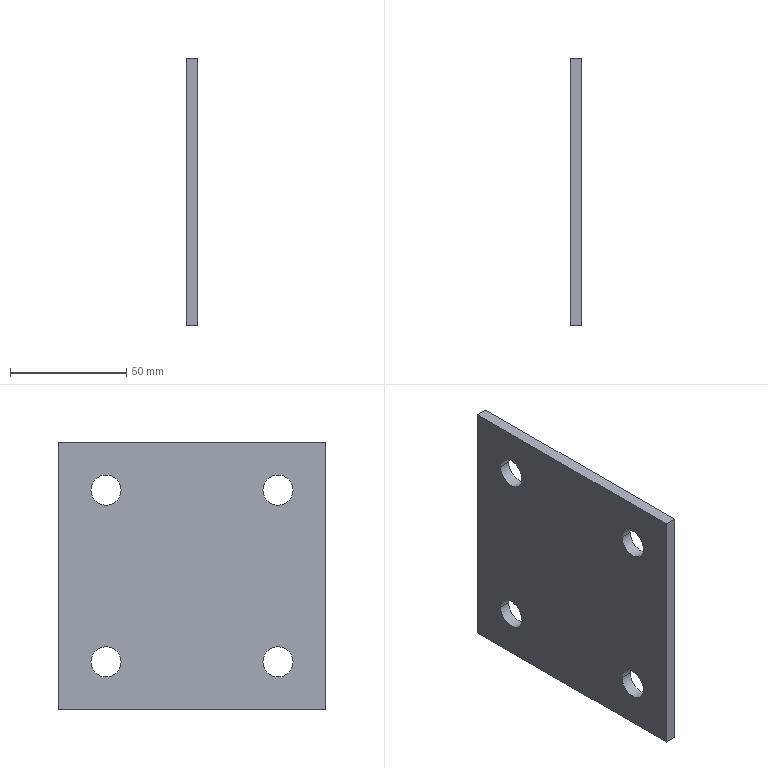Part | STEP file | 09-38 Cylinder pad plate | 1 solid | 14 faces | box 5 x 115 x 115 mm | volume 63470 mm3 | cylinder 8 | plane 6 | commonest cylinder face diameters 13 x8
STEP:
#1=CARTESIAN_POINT('',(0.,0.,0.));
#2=DIRECTION('',(0.,0.,1.));
#3=DIRECTION('',(1.,0.,0.));
#4=AXIS2_PLACEMENT_3D('',#1,#2,#3);
#5=CARTESIAN_POINT('',(5.,-43.5,37.));
#6=VERTEX_POINT('',#5);
#7=CARTESIAN_POINT('',(0.,-43.5,37.));
#8=VERTEX_POINT('',#7);
#9=CARTESIAN_POINT('',(5.,-43.5,37.));
#10=DIRECTION('',(-1.,0.,0.));
#11=VECTOR('',#10,1.);
#12=LINE('',#9,#11);
#13=CARTESIAN_POINT('',(5.,-37.,37.));
#14=DIRECTION('',(-1.,0.,0.));
#15=DIRECTION('',(0.,-1.,0.));
#16=AXIS2_PLACEMENT_3D('',#13,#14,#15);
#17=CYLINDRICAL_SURFACE('',#16,6.5);
#18=CARTESIAN_POINT('',(6.283,0.));
#19=DIRECTION('',(0.,1.));
#20=VECTOR('',#19,1.);
#21=LINE('',#18,#20);
#22=(GEOMETRIC_REPRESENTATION_CONTEXT(2)PARAMETRIC_REPRESENTATION_CONTEXT()REPRESENTATION_CONTEXT('',''));
#23=DEFINITIONAL_REPRESENTATION('',(#21),#22);
#24=PCURVE('',#17,#23);
#25=CARTESIAN_POINT('',(5.,-37.,37.));
#26=DIRECTION('',(-1.,0.,0.));
#27=DIRECTION('',(0.,-1.,0.));
#28=AXIS2_PLACEMENT_3D('',#25,#26,#27);
#29=CYLINDRICAL_SURFACE('',#28,6.5);
#30=CARTESIAN_POINT('',(0.,0.));
#31=DIRECTION('',(0.,1.));
#32=VECTOR('',#31,1.);
#33=LINE('',#30,#32);
#34=(GEOMETRIC_REPRESENTATION_CONTEXT(2)PARAMETRIC_REPRESENTATION_CONTEXT()REPRESENTATION_CONTEXT('',''));
#35=DEFINITIONAL_REPRESENTATION('',(#33),#34);
#36=PCURVE('',#29,#35);
#37=SURFACE_CURVE('',#12,(#24,#36),.PCURVE_S1.);
#38=EDGE_CURVE('',#6,#8,#37,.T.);
#39=ORIENTED_EDGE('',*,*,#38,.T.);
#40=CARTESIAN_POINT('',(0.,-30.5,37.));
#41=VERTEX_POINT('',#40);
#42=CARTESIAN_POINT('',(0.,-37.,37.));
#43=DIRECTION('',(-1.,0.,0.));
#44=DIRECTION('',(0.,-1.,0.));
#45=AXIS2_PLACEMENT_3D('',#42,#43,#44);
#46=CIRCLE('',#45,6.5);
#47=CARTESIAN_POINT('',(0.,5.));
#48=DIRECTION('',(1.,0.));
#49=VECTOR('',#48,1.);
#50=LINE('',#47,#49);
#51=(GEOMETRIC_REPRESENTATION_CONTEXT(2)PARAMETRIC_REPRESENTATION_CONTEXT()REPRESENTATION_CONTEXT('',''));
#52=DEFINITIONAL_REPRESENTATION('',(#50),#51);
#53=PCURVE('',#17,#52);
#54=CARTESIAN_POINT('',(0.,-57.5,-57.5));
#55=DIRECTION('',(-1.,0.,0.));
#56=DIRECTION('',(0.,0.,1.));
#57=AXIS2_PLACEMENT_3D('',#54,#55,#56);
#58=PLANE('',#57);
#59=CARTESIAN_POINT('',(94.5,20.5));
#60=DIRECTION('',(0.,-1.));
#61=AXIS2_PLACEMENT_2D('',#59,#60);
#62=CIRCLE('',#61,6.5);
#63=(GEOMETRIC_REPRESENTATION_CONTEXT(2)PARAMETRIC_REPRESENTATION_CONTEXT()REPRESENTATION_CONTEXT('',''));
#64=DEFINITIONAL_REPRESENTATION('',(#62),#63);
#65=PCURVE('',#58,#64);
#66=SURFACE_CURVE('',#46,(#53,#65),.PCURVE_S1.);
#67=EDGE_CURVE('',#41,#8,#66,.T.);
#68=ORIENTED_EDGE('',*,*,#67,.F.);
#69=CARTESIAN_POINT('',(5.,-30.5,37.));
#70=VERTEX_POINT('',#69);
#71=CARTESIAN_POINT('',(5.,-30.5,37.));
#72=DIRECTION('',(-1.,0.,0.));
#73=VECTOR('',#72,1.);
#74=LINE('',#71,#73);
#75=CARTESIAN_POINT('',(3.142,0.));
#76=DIRECTION('',(0.,1.));
#77=VECTOR('',#76,1.);
#78=LINE('',#75,#77);
#79=(GEOMETRIC_REPRESENTATION_CONTEXT(2)PARAMETRIC_REPRESENTATION_CONTEXT()REPRESENTATION_CONTEXT('',''));
#80=DEFINITIONAL_REPRESENTATION('',(#78),#79);
#81=PCURVE('',#17,#80);
#82=CARTESIAN_POINT('',(3.142,0.));
#83=DIRECTION('',(0.,1.));
#84=VECTOR('',#83,1.);
#85=LINE('',#82,#84);
#86=(GEOMETRIC_REPRESENTATION_CONTEXT(2)PARAMETRIC_REPRESENTATION_CONTEXT()REPRESENTATION_CONTEXT('',''));
#87=DEFINITIONAL_REPRESENTATION('',(#85),#86);
#88=PCURVE('',#29,#87);
#89=SURFACE_CURVE('',#74,(#81,#88),.PCURVE_S1.);
#90=EDGE_CURVE('',#70,#41,#89,.T.);
#91=ORIENTED_EDGE('',*,*,#90,.F.);
#92=CARTESIAN_POINT('',(5.,-37.,37.));
#93=DIRECTION('',(1.,0.,0.));
#94=DIRECTION('',(0.,-1.,0.));
#95=AXIS2_PLACEMENT_3D('',#92,#93,#94);
#96=CIRCLE('',#95,6.5);
#97=CARTESIAN_POINT('',(6.283,0.));
#98=DIRECTION('',(-1.,0.));
#99=VECTOR('',#98,1.);
#100=LINE('',#97,#99);
#101=(GEOMETRIC_REPRESENTATION_CONTEXT(2)PARAMETRIC_REPRESENTATION_CONTEXT()REPRESENTATION_CONTEXT('',''));
#102=DEFINITIONAL_REPRESENTATION('',(#100),#101);
#103=PCURVE('',#17,#102);
#104=CARTESIAN_POINT('',(5.,-57.5,-57.5));
#105=DIRECTION('',(-1.,0.,0.));
#106=DIRECTION('',(0.,0.,1.));
#107=AXIS2_PLACEMENT_3D('',#104,#105,#106);
#108=PLANE('',#107);
#109=CARTESIAN_POINT('',(94.5,14.));
#110=CARTESIAN_POINT('',(83.242,14.));
#111=CARTESIAN_POINT('',(88.871,23.75));
#112=CARTESIAN_POINT('',(94.5,33.5));
#113=CARTESIAN_POINT('',(100.129,23.75));
#114=CARTESIAN_POINT('',(105.758,14.));
#115=CARTESIAN_POINT('',(94.5,14.));
#116=(BOUNDED_CURVE()B_SPLINE_CURVE(2,(#109,#110,#111,#112,#113,#114,#115),.UNSPECIFIED.,.T.,.F.)B_SPLINE_CURVE_WITH_KNOTS((1,2,2,2,2,1),(-2.094,0.,2.094,4.189,6.283,8.378),.UNSPECIFIED.)CURVE()GEOMETRIC_REPRESENTATION_ITEM()RATIONAL_B_SPLINE_CURVE((1.,0.5,1.,0.5,1.,0.5,1.))REPRESENTATION_ITEM(''));
#117=(GEOMETRIC_REPRESENTATION_CONTEXT(2)PARAMETRIC_REPRESENTATION_CONTEXT()REPRESENTATION_CONTEXT('',''));
#118=DEFINITIONAL_REPRESENTATION('',(#116),#117);
#119=PCURVE('',#108,#118);
#120=SURFACE_CURVE('',#96,(#103,#119),.PCURVE_S1.);
#121=EDGE_CURVE('',#6,#70,#120,.T.);
#122=ORIENTED_EDGE('',*,*,#121,.F.);
#123=EDGE_LOOP('',(#39,#68,#91,#122));
#124=FACE_BOUND('',#123,.F.);
#125=ADVANCED_FACE('',(#124),#17,.F.);
#126=CARTESIAN_POINT('',(5.,30.5,-37.));
#127=VERTEX_POINT('',#126);
#128=CARTESIAN_POINT('',(0.,30.5,-37.));
#129=VERTEX_POINT('',#128);
#130=CARTESIAN_POINT('',(5.,30.5,-37.));
#131=DIRECTION('',(-1.,0.,0.));
#132=VECTOR('',#131,1.);
#133=LINE('',#130,#132);
#134=CARTESIAN_POINT('',(5.,37.,-37.));
#135=DIRECTION('',(-1.,0.,0.));
#136=DIRECTION('',(0.,-1.,0.));
#137=AXIS2_PLACEMENT_3D('',#134,#135,#136);
#138=CYLINDRICAL_SURFACE('',#137,6.5);
#139=CARTESIAN_POINT('',(6.283,0.));
#140=DIRECTION('',(0.,1.));
#141=VECTOR('',#140,1.);
#142=LINE('',#139,#141);
#143=(GEOMETRIC_REPRESENTATION_CONTEXT(2)PARAMETRIC_REPRESENTATION_CONTEXT()REPRESENTATION_CONTEXT('',''));
#144=DEFINITIONAL_REPRESENTATION('',(#142),#143);
#145=PCURVE('',#138,#144);
#146=CARTESIAN_POINT('',(5.,37.,-37.));
#147=DIRECTION('',(-1.,0.,0.));
#148=DIRECTION('',(0.,-1.,0.));
#149=AXIS2_PLACEMENT_3D('',#146,#147,#148);
#150=CYLINDRICAL_SURFACE('',#149,6.5);
#151=CARTESIAN_POINT('',(0.,0.));
#152=DIRECTION('',(0.,1.));
#153=VECTOR('',#152,1.);
#154=LINE('',#151,#153);
#155=(GEOMETRIC_REPRESENTATION_CONTEXT(2)PARAMETRIC_REPRESENTATION_CONTEXT()REPRESENTATION_CONTEXT('',''));
#156=DEFINITIONAL_REPRESENTATION('',(#154),#155);
#157=PCURVE('',#150,#156);
#158=SURFACE_CURVE('',#133,(#145,#157),.PCURVE_S1.);
#159=EDGE_CURVE('',#127,#129,#158,.T.);
#160=ORIENTED_EDGE('',*,*,#159,.T.);
#161=CARTESIAN_POINT('',(0.,43.5,-37.));
#162=VERTEX_POINT('',#161);
#163=CARTESIAN_POINT('',(0.,37.,-37.));
#164=DIRECTION('',(1.,0.,0.));
#165=DIRECTION('',(0.,-1.,0.));
#166=AXIS2_PLACEMENT_3D('',#163,#164,#165);
#167=CIRCLE('',#166,6.5);
#168=CARTESIAN_POINT('',(6.283,5.));
#169=DIRECTION('',(-1.,0.));
#170=VECTOR('',#169,1.);
#171=LINE('',#168,#170);
#172=(GEOMETRIC_REPRESENTATION_CONTEXT(2)PARAMETRIC_REPRESENTATION_CONTEXT()REPRESENTATION_CONTEXT('',''));
#173=DEFINITIONAL_REPRESENTATION('',(#171),#172);
#174=PCURVE('',#138,#173);
#175=CARTESIAN_POINT('',(20.5,88.));
#176=CARTESIAN_POINT('',(9.242,88.));
#177=CARTESIAN_POINT('',(14.871,97.75));
#178=CARTESIAN_POINT('',(20.5,107.5));
#179=CARTESIAN_POINT('',(26.129,97.75));
#180=CARTESIAN_POINT('',(31.758,88.));
#181=CARTESIAN_POINT('',(20.5,88.));
#182=(BOUNDED_CURVE()B_SPLINE_CURVE(2,(#175,#176,#177,#178,#179,#180,#181),.UNSPECIFIED.,.T.,.F.)B_SPLINE_CURVE_WITH_KNOTS((1,2,2,2,2,1),(-2.094,0.,2.094,4.189,6.283,8.378),.UNSPECIFIED.)CURVE()GEOMETRIC_REPRESENTATION_ITEM()RATIONAL_B_SPLINE_CURVE((1.,0.5,1.,0.5,1.,0.5,1.))REPRESENTATION_ITEM(''));
#183=(GEOMETRIC_REPRESENTATION_CONTEXT(2)PARAMETRIC_REPRESENTATION_CONTEXT()REPRESENTATION_CONTEXT('',''));
#184=DEFINITIONAL_REPRESENTATION('',(#182),#183);
#185=PCURVE('',#58,#184);
#186=SURFACE_CURVE('',#167,(#174,#185),.PCURVE_S1.);
#187=EDGE_CURVE('',#129,#162,#186,.T.);
#188=ORIENTED_EDGE('',*,*,#187,.T.);
#189=CARTESIAN_POINT('',(5.,43.5,-37.));
#190=VERTEX_POINT('',#189);
#191=CARTESIAN_POINT('',(5.,43.5,-37.));
#192=DIRECTION('',(-1.,0.,0.));
#193=VECTOR('',#192,1.);
#194=LINE('',#191,#193);
#195=CARTESIAN_POINT('',(3.142,0.));
#196=DIRECTION('',(0.,1.));
#197=VECTOR('',#196,1.);
#198=LINE('',#195,#197);
#199=(GEOMETRIC_REPRESENTATION_CONTEXT(2)PARAMETRIC_REPRESENTATION_CONTEXT()REPRESENTATION_CONTEXT('',''));
#200=DEFINITIONAL_REPRESENTATION('',(#198),#199);
#201=PCURVE('',#138,#200);
#202=CARTESIAN_POINT('',(3.142,0.));
#203=DIRECTION('',(0.,1.));
#204=VECTOR('',#203,1.);
#205=LINE('',#202,#204);
#206=(GEOMETRIC_REPRESENTATION_CONTEXT(2)PARAMETRIC_REPRESENTATION_CONTEXT()REPRESENTATION_CONTEXT('',''));
#207=DEFINITIONAL_REPRESENTATION('',(#205),#206);
#208=PCURVE('',#150,#207);
#209=SURFACE_CURVE('',#194,(#201,#208),.PCURVE_S1.);
#210=EDGE_CURVE('',#190,#162,#209,.T.);
#211=ORIENTED_EDGE('',*,*,#210,.F.);
#212=CARTESIAN_POINT('',(5.,37.,-37.));
#213=DIRECTION('',(1.,0.,0.));
#214=DIRECTION('',(0.,-1.,0.));
#215=AXIS2_PLACEMENT_3D('',#212,#213,#214);
#216=CIRCLE('',#215,6.5);
#217=CARTESIAN_POINT('',(6.283,0.));
#218=DIRECTION('',(-1.,0.));
#219=VECTOR('',#218,1.);
#220=LINE('',#217,#219);
#221=(GEOMETRIC_REPRESENTATION_CONTEXT(2)PARAMETRIC_REPRESENTATION_CONTEXT()REPRESENTATION_CONTEXT('',''));
#222=DEFINITIONAL_REPRESENTATION('',(#220),#221);
#223=PCURVE('',#138,#222);
#224=CARTESIAN_POINT('',(20.5,88.));
#225=CARTESIAN_POINT('',(9.242,88.));
#226=CARTESIAN_POINT('',(14.871,97.75));
#227=CARTESIAN_POINT('',(20.5,107.5));
#228=CARTESIAN_POINT('',(26.129,97.75));
#229=CARTESIAN_POINT('',(31.758,88.));
#230=CARTESIAN_POINT('',(20.5,88.));
#231=(BOUNDED_CURVE()B_SPLINE_CURVE(2,(#224,#225,#226,#227,#228,#229,#230),.UNSPECIFIED.,.T.,.F.)B_SPLINE_CURVE_WITH_KNOTS((1,2,2,2,2,1),(-2.094,0.,2.094,4.189,6.283,8.378),.UNSPECIFIED.)CURVE()GEOMETRIC_REPRESENTATION_ITEM()RATIONAL_B_SPLINE_CURVE((1.,0.5,1.,0.5,1.,0.5,1.))REPRESENTATION_ITEM(''));
#232=(GEOMETRIC_REPRESENTATION_CONTEXT(2)PARAMETRIC_REPRESENTATION_CONTEXT()REPRESENTATION_CONTEXT('',''));
#233=DEFINITIONAL_REPRESENTATION('',(#231),#232);
#234=PCURVE('',#108,#233);
#235=SURFACE_CURVE('',#216,(#223,#234),.PCURVE_S1.);
#236=EDGE_CURVE('',#127,#190,#235,.T.);
#237=ORIENTED_EDGE('',*,*,#236,.F.);
#238=EDGE_LOOP('',(#160,#188,#211,#237));
#239=FACE_BOUND('',#238,.F.);
#240=ADVANCED_FACE('',(#239),#138,.F.);
#241=CARTESIAN_POINT('',(5.,30.5,37.));
#242=VERTEX_POINT('',#241);
#243=CARTESIAN_POINT('',(0.,30.5,37.));
#244=VERTEX_POINT('',#243);
#245=CARTESIAN_POINT('',(5.,30.5,37.));
#246=DIRECTION('',(-1.,0.,0.));
#247=VECTOR('',#246,1.);
#248=LINE('',#245,#247);
#249=CARTESIAN_POINT('',(5.,37.,37.));
#250=DIRECTION('',(-1.,0.,0.));
#251=DIRECTION('',(0.,-1.,0.));
#252=AXIS2_PLACEMENT_3D('',#249,#250,#251);
#253=CYLINDRICAL_SURFACE('',#252,6.5);
#254=CARTESIAN_POINT('',(6.283,0.));
#255=DIRECTION('',(0.,1.));
#256=VECTOR('',#255,1.);
#257=LINE('',#254,#256);
#258=(GEOMETRIC_REPRESENTATION_CONTEXT(2)PARAMETRIC_REPRESENTATION_CONTEXT()REPRESENTATION_CONTEXT('',''));
#259=DEFINITIONAL_REPRESENTATION('',(#257),#258);
#260=PCURVE('',#253,#259);
#261=CARTESIAN_POINT('',(5.,37.,37.));
#262=DIRECTION('',(-1.,0.,0.));
#263=DIRECTION('',(0.,-1.,0.));
#264=AXIS2_PLACEMENT_3D('',#261,#262,#263);
#265=CYLINDRICAL_SURFACE('',#264,6.5);
#266=CARTESIAN_POINT('',(0.,0.));
#267=DIRECTION('',(0.,1.));
#268=VECTOR('',#267,1.);
#269=LINE('',#266,#268);
#270=(GEOMETRIC_REPRESENTATION_CONTEXT(2)PARAMETRIC_REPRESENTATION_CONTEXT()REPRESENTATION_CONTEXT('',''));
#271=DEFINITIONAL_REPRESENTATION('',(#269),#270);
#272=PCURVE('',#265,#271);
#273=SURFACE_CURVE('',#248,(#260,#272),.PCURVE_S1.);
#274=EDGE_CURVE('',#242,#244,#273,.T.);
#275=ORIENTED_EDGE('',*,*,#274,.T.);
#276=CARTESIAN_POINT('',(0.,43.5,37.));
#277=VERTEX_POINT('',#276);
#278=CARTESIAN_POINT('',(0.,37.,37.));
#279=DIRECTION('',(1.,0.,0.));
#280=DIRECTION('',(0.,-1.,0.));
#281=AXIS2_PLACEMENT_3D('',#278,#279,#280);
#282=CIRCLE('',#281,6.5);
#283=CARTESIAN_POINT('',(6.283,5.));
#284=DIRECTION('',(-1.,0.));
#285=VECTOR('',#284,1.);
#286=LINE('',#283,#285);
#287=(GEOMETRIC_REPRESENTATION_CONTEXT(2)PARAMETRIC_REPRESENTATION_CONTEXT()REPRESENTATION_CONTEXT('',''));
#288=DEFINITIONAL_REPRESENTATION('',(#286),#287);
#289=PCURVE('',#253,#288);
#290=CARTESIAN_POINT('',(94.5,88.));
#291=CARTESIAN_POINT('',(83.242,88.));
#292=CARTESIAN_POINT('',(88.871,97.75));
#293=CARTESIAN_POINT('',(94.5,107.5));
#294=CARTESIAN_POINT('',(100.129,97.75));
#295=CARTESIAN_POINT('',(105.758,88.));
#296=CARTESIAN_POINT('',(94.5,88.));
#297=(BOUNDED_CURVE()B_SPLINE_CURVE(2,(#290,#291,#292,#293,#294,#295,#296),.UNSPECIFIED.,.T.,.F.)B_SPLINE_CURVE_WITH_KNOTS((1,2,2,2,2,1),(-2.094,0.,2.094,4.189,6.283,8.378),.UNSPECIFIED.)CURVE()GEOMETRIC_REPRESENTATION_ITEM()RATIONAL_B_SPLINE_CURVE((1.,0.5,1.,0.5,1.,0.5,1.))REPRESENTATION_ITEM(''));
#298=(GEOMETRIC_REPRESENTATION_CONTEXT(2)PARAMETRIC_REPRESENTATION_CONTEXT()REPRESENTATION_CONTEXT('',''));
#299=DEFINITIONAL_REPRESENTATION('',(#297),#298);
#300=PCURVE('',#58,#299);
#301=SURFACE_CURVE('',#282,(#289,#300),.PCURVE_S1.);
#302=EDGE_CURVE('',#244,#277,#301,.T.);
#303=ORIENTED_EDGE('',*,*,#302,.T.);
#304=CARTESIAN_POINT('',(5.,43.5,37.));
#305=VERTEX_POINT('',#304);
#306=CARTESIAN_POINT('',(5.,43.5,37.));
#307=DIRECTION('',(-1.,0.,0.));
#308=VECTOR('',#307,1.);
#309=LINE('',#306,#308);
#310=CARTESIAN_POINT('',(3.142,0.));
#311=DIRECTION('',(0.,1.));
#312=VECTOR('',#311,1.);
#313=LINE('',#310,#312);
#314=(GEOMETRIC_REPRESENTATION_CONTEXT(2)PARAMETRIC_REPRESENTATION_CONTEXT()REPRESENTATION_CONTEXT('',''));
#315=DEFINITIONAL_REPRESENTATION('',(#313),#314);
#316=PCURVE('',#253,#315);
#317=CARTESIAN_POINT('',(3.142,0.));
#318=DIRECTION('',(0.,1.));
#319=VECTOR('',#318,1.);
#320=LINE('',#317,#319);
#321=(GEOMETRIC_REPRESENTATION_CONTEXT(2)PARAMETRIC_REPRESENTATION_CONTEXT()REPRESENTATION_CONTEXT('',''));
#322=DEFINITIONAL_REPRESENTATION('',(#320),#321);
#323=PCURVE('',#265,#322);
#324=SURFACE_CURVE('',#309,(#316,#323),.PCURVE_S1.);
#325=EDGE_CURVE('',#305,#277,#324,.T.);
#326=ORIENTED_EDGE('',*,*,#325,.F.);
#327=CARTESIAN_POINT('',(5.,37.,37.));
#328=DIRECTION('',(1.,0.,0.));
#329=DIRECTION('',(0.,-1.,0.));
#330=AXIS2_PLACEMENT_3D('',#327,#328,#329);
#331=CIRCLE('',#330,6.5);
#332=CARTESIAN_POINT('',(6.283,0.));
#333=DIRECTION('',(-1.,0.));
#334=VECTOR('',#333,1.);
#335=LINE('',#332,#334);
#336=(GEOMETRIC_REPRESENTATION_CONTEXT(2)PARAMETRIC_REPRESENTATION_CONTEXT()REPRESENTATION_CONTEXT('',''));
#337=DEFINITIONAL_REPRESENTATION('',(#335),#336);
#338=PCURVE('',#253,#337);
#339=CARTESIAN_POINT('',(94.5,88.));
#340=CARTESIAN_POINT('',(83.242,88.));
#341=CARTESIAN_POINT('',(88.871,97.75));
#342=CARTESIAN_POINT('',(94.5,107.5));
#343=CARTESIAN_POINT('',(100.129,97.75));
#344=CARTESIAN_POINT('',(105.758,88.));
#345=CARTESIAN_POINT('',(94.5,88.));
#346=(BOUNDED_CURVE()B_SPLINE_CURVE(2,(#339,#340,#341,#342,#343,#344,#345),.UNSPECIFIED.,.T.,.F.)B_SPLINE_CURVE_WITH_KNOTS((1,2,2,2,2,1),(-2.094,0.,2.094,4.189,6.283,8.378),.UNSPECIFIED.)CURVE()GEOMETRIC_REPRESENTATION_ITEM()RATIONAL_B_SPLINE_CURVE((1.,0.5,1.,0.5,1.,0.5,1.))REPRESENTATION_ITEM(''));
#347=(GEOMETRIC_REPRESENTATION_CONTEXT(2)PARAMETRIC_REPRESENTATION_CONTEXT()REPRESENTATION_CONTEXT('',''));
#348=DEFINITIONAL_REPRESENTATION('',(#346),#347);
#349=PCURVE('',#108,#348);
#350=SURFACE_CURVE('',#331,(#338,#349),.PCURVE_S1.);
#351=EDGE_CURVE('',#242,#305,#350,.T.);
#352=ORIENTED_EDGE('',*,*,#351,.F.);
#353=EDGE_LOOP('',(#275,#303,#326,#352));
#354=FACE_BOUND('',#353,.F.);
#355=ADVANCED_FACE('',(#354),#253,.F.);
#356=CARTESIAN_POINT('',(5.,-43.5,-37.));
#357=VERTEX_POINT('',#356);
#358=CARTESIAN_POINT('',(0.,-43.5,-37.));
#359=VERTEX_POINT('',#358);
#360=CARTESIAN_POINT('',(5.,-43.5,-37.));
#361=DIRECTION('',(-1.,0.,0.));
#362=VECTOR('',#361,1.);
#363=LINE('',#360,#362);
#364=CARTESIAN_POINT('',(5.,-37.,-37.));
#365=DIRECTION('',(-1.,0.,0.));
#366=DIRECTION('',(0.,-1.,0.));
#367=AXIS2_PLACEMENT_3D('',#364,#365,#366);
#368=CYLINDRICAL_SURFACE('',#367,6.5);
#369=CARTESIAN_POINT('',(6.283,0.));
#370=DIRECTION('',(0.,1.));
#371=VECTOR('',#370,1.);
#372=LINE('',#369,#371);
#373=(GEOMETRIC_REPRESENTATION_CONTEXT(2)PARAMETRIC_REPRESENTATION_CONTEXT()REPRESENTATION_CONTEXT('',''));
#374=DEFINITIONAL_REPRESENTATION('',(#372),#373);
#375=PCURVE('',#368,#374);
#376=CARTESIAN_POINT('',(5.,-37.,-37.));
#377=DIRECTION('',(-1.,0.,0.));
#378=DIRECTION('',(0.,-1.,0.));
#379=AXIS2_PLACEMENT_3D('',#376,#377,#378);
#380=CYLINDRICAL_SURFACE('',#379,6.5);
#381=CARTESIAN_POINT('',(0.,0.));
#382=DIRECTION('',(0.,1.));
#383=VECTOR('',#382,1.);
#384=LINE('',#381,#383);
#385=(GEOMETRIC_REPRESENTATION_CONTEXT(2)PARAMETRIC_REPRESENTATION_CONTEXT()REPRESENTATION_CONTEXT('',''));
#386=DEFINITIONAL_REPRESENTATION('',(#384),#385);
#387=PCURVE('',#380,#386);
#388=SURFACE_CURVE('',#363,(#375,#387),.PCURVE_S1.);
#389=EDGE_CURVE('',#357,#359,#388,.T.);
#390=ORIENTED_EDGE('',*,*,#389,.T.);
#391=CARTESIAN_POINT('',(0.,-30.5,-37.));
#392=VERTEX_POINT('',#391);
#393=CARTESIAN_POINT('',(0.,-37.,-37.));
#394=DIRECTION('',(1.,0.,0.));
#395=DIRECTION('',(0.,-1.,0.));
#396=AXIS2_PLACEMENT_3D('',#393,#394,#395);
#397=CIRCLE('',#396,6.5);
#398=CARTESIAN_POINT('',(6.283,5.));
#399=DIRECTION('',(-1.,0.));
#400=VECTOR('',#399,1.);
#401=LINE('',#398,#400);
#402=(GEOMETRIC_REPRESENTATION_CONTEXT(2)PARAMETRIC_REPRESENTATION_CONTEXT()REPRESENTATION_CONTEXT('',''));
#403=DEFINITIONAL_REPRESENTATION('',(#401),#402);
#404=PCURVE('',#368,#403);
#405=CARTESIAN_POINT('',(20.5,14.));
#406=CARTESIAN_POINT('',(9.242,14.));
#407=CARTESIAN_POINT('',(14.871,23.75));
#408=CARTESIAN_POINT('',(20.5,33.5));
#409=CARTESIAN_POINT('',(26.129,23.75));
#410=CARTESIAN_POINT('',(31.758,14.));
#411=CARTESIAN_POINT('',(20.5,14.));
#412=(BOUNDED_CURVE()B_SPLINE_CURVE(2,(#405,#406,#407,#408,#409,#410,#411),.UNSPECIFIED.,.T.,.F.)B_SPLINE_CURVE_WITH_KNOTS((1,2,2,2,2,1),(-2.094,0.,2.094,4.189,6.283,8.378),.UNSPECIFIED.)CURVE()GEOMETRIC_REPRESENTATION_ITEM()RATIONAL_B_SPLINE_CURVE((1.,0.5,1.,0.5,1.,0.5,1.))REPRESENTATION_ITEM(''));
#413=(GEOMETRIC_REPRESENTATION_CONTEXT(2)PARAMETRIC_REPRESENTATION_CONTEXT()REPRESENTATION_CONTEXT('',''));
#414=DEFINITIONAL_REPRESENTATION('',(#412),#413);
#415=PCURVE('',#58,#414);
#416=SURFACE_CURVE('',#397,(#404,#415),.PCURVE_S1.);
#417=EDGE_CURVE('',#359,#392,#416,.T.);
#418=ORIENTED_EDGE('',*,*,#417,.T.);
#419=CARTESIAN_POINT('',(5.,-30.5,-37.));
#420=VERTEX_POINT('',#419);
#421=CARTESIAN_POINT('',(5.,-30.5,-37.));
#422=DIRECTION('',(-1.,0.,0.));
#423=VECTOR('',#422,1.);
#424=LINE('',#421,#423);
#425=CARTESIAN_POINT('',(3.142,0.));
#426=DIRECTION('',(0.,1.));
#427=VECTOR('',#426,1.);
#428=LINE('',#425,#427);
#429=(GEOMETRIC_REPRESENTATION_CONTEXT(2)PARAMETRIC_REPRESENTATION_CONTEXT()REPRESENTATION_CONTEXT('',''));
#430=DEFINITIONAL_REPRESENTATION('',(#428),#429);
#431=PCURVE('',#368,#430);
#432=CARTESIAN_POINT('',(3.142,0.));
#433=DIRECTION('',(0.,1.));
#434=VECTOR('',#433,1.);
#435=LINE('',#432,#434);
#436=(GEOMETRIC_REPRESENTATION_CONTEXT(2)PARAMETRIC_REPRESENTATION_CONTEXT()REPRESENTATION_CONTEXT('',''));
#437=DEFINITIONAL_REPRESENTATION('',(#435),#436);
#438=PCURVE('',#380,#437);
#439=SURFACE_CURVE('',#424,(#431,#438),.PCURVE_S1.);
#440=EDGE_CURVE('',#420,#392,#439,.T.);
#441=ORIENTED_EDGE('',*,*,#440,.F.);
#442=CARTESIAN_POINT('',(5.,-37.,-37.));
#443=DIRECTION('',(1.,0.,0.));
#444=DIRECTION('',(0.,-1.,0.));
#445=AXIS2_PLACEMENT_3D('',#442,#443,#444);
#446=CIRCLE('',#445,6.5);
#447=CARTESIAN_POINT('',(6.283,0.));
#448=DIRECTION('',(-1.,0.));
#449=VECTOR('',#448,1.);
#450=LINE('',#447,#449);
#451=(GEOMETRIC_REPRESENTATION_CONTEXT(2)PARAMETRIC_REPRESENTATION_CONTEXT()REPRESENTATION_CONTEXT('',''));
#452=DEFINITIONAL_REPRESENTATION('',(#450),#451);
#453=PCURVE('',#368,#452);
#454=CARTESIAN_POINT('',(20.5,14.));
#455=CARTESIAN_POINT('',(9.242,14.));
#456=CARTESIAN_POINT('',(14.871,23.75));
#457=CARTESIAN_POINT('',(20.5,33.5));
#458=CARTESIAN_POINT('',(26.129,23.75));
#459=CARTESIAN_POINT('',(31.758,14.));
#460=CARTESIAN_POINT('',(20.5,14.));
#461=(BOUNDED_CURVE()B_SPLINE_CURVE(2,(#454,#455,#456,#457,#458,#459,#460),.UNSPECIFIED.,.T.,.F.)B_SPLINE_CURVE_WITH_KNOTS((1,2,2,2,2,1),(-2.094,0.,2.094,4.189,6.283,8.378),.UNSPECIFIED.)CURVE()GEOMETRIC_REPRESENTATION_ITEM()RATIONAL_B_SPLINE_CURVE((1.,0.5,1.,0.5,1.,0.5,1.))REPRESENTATION_ITEM(''));
#462=(GEOMETRIC_REPRESENTATION_CONTEXT(2)PARAMETRIC_REPRESENTATION_CONTEXT()REPRESENTATION_CONTEXT('',''));
#463=DEFINITIONAL_REPRESENTATION('',(#461),#462);
#464=PCURVE('',#108,#463);
#465=SURFACE_CURVE('',#446,(#453,#464),.PCURVE_S1.);
#466=EDGE_CURVE('',#357,#420,#465,.T.);
#467=ORIENTED_EDGE('',*,*,#466,.F.);
#468=EDGE_LOOP('',(#390,#418,#441,#467));
#469=FACE_BOUND('',#468,.F.);
#470=ADVANCED_FACE('',(#469),#368,.F.);
#471=CARTESIAN_POINT('',(0.,-37.,37.));
#472=DIRECTION('',(-1.,0.,0.));
#473=DIRECTION('',(0.,-1.,0.));
#474=AXIS2_PLACEMENT_3D('',#471,#472,#473);
#475=CIRCLE('',#474,6.5);
#476=CARTESIAN_POINT('',(0.,5.));
#477=DIRECTION('',(1.,0.));
#478=VECTOR('',#477,1.);
#479=LINE('',#476,#478);
#480=(GEOMETRIC_REPRESENTATION_CONTEXT(2)PARAMETRIC_REPRESENTATION_CONTEXT()REPRESENTATION_CONTEXT('',''));
#481=DEFINITIONAL_REPRESENTATION('',(#479),#480);
#482=PCURVE('',#29,#481);
#483=CARTESIAN_POINT('',(94.5,20.5));
#484=DIRECTION('',(0.,-1.));
#485=AXIS2_PLACEMENT_2D('',#483,#484);
#486=CIRCLE('',#485,6.5);
#487=(GEOMETRIC_REPRESENTATION_CONTEXT(2)PARAMETRIC_REPRESENTATION_CONTEXT()REPRESENTATION_CONTEXT('',''));
#488=DEFINITIONAL_REPRESENTATION('',(#486),#487);
#489=PCURVE('',#58,#488);
#490=SURFACE_CURVE('',#475,(#482,#489),.PCURVE_S1.);
#491=EDGE_CURVE('',#8,#41,#490,.T.);
#492=ORIENTED_EDGE('',*,*,#491,.F.);
#493=ORIENTED_EDGE('',*,*,#38,.F.);
#494=CARTESIAN_POINT('',(5.,-37.,37.));
#495=DIRECTION('',(1.,0.,0.));
#496=DIRECTION('',(0.,-1.,0.));
#497=AXIS2_PLACEMENT_3D('',#494,#495,#496);
#498=CIRCLE('',#497,6.5);
#499=CARTESIAN_POINT('',(6.283,0.));
#500=DIRECTION('',(-1.,0.));
#501=VECTOR('',#500,1.);
#502=LINE('',#499,#501);
#503=(GEOMETRIC_REPRESENTATION_CONTEXT(2)PARAMETRIC_REPRESENTATION_CONTEXT()REPRESENTATION_CONTEXT('',''));
#504=DEFINITIONAL_REPRESENTATION('',(#502),#503);
#505=PCURVE('',#29,#504);
#506=CARTESIAN_POINT('',(94.5,14.));
#507=CARTESIAN_POINT('',(83.242,14.));
#508=CARTESIAN_POINT('',(88.871,23.75));
#509=CARTESIAN_POINT('',(94.5,33.5));
#510=CARTESIAN_POINT('',(100.129,23.75));
#511=CARTESIAN_POINT('',(105.758,14.));
#512=CARTESIAN_POINT('',(94.5,14.));
#513=(BOUNDED_CURVE()B_SPLINE_CURVE(2,(#506,#507,#508,#509,#510,#511,#512),.UNSPECIFIED.,.T.,.F.)B_SPLINE_CURVE_WITH_KNOTS((1,2,2,2,2,1),(-2.094,0.,2.094,4.189,6.283,8.378),.UNSPECIFIED.)CURVE()GEOMETRIC_REPRESENTATION_ITEM()RATIONAL_B_SPLINE_CURVE((1.,0.5,1.,0.5,1.,0.5,1.))REPRESENTATION_ITEM(''));
#514=(GEOMETRIC_REPRESENTATION_CONTEXT(2)PARAMETRIC_REPRESENTATION_CONTEXT()REPRESENTATION_CONTEXT('',''));
#515=DEFINITIONAL_REPRESENTATION('',(#513),#514);
#516=PCURVE('',#108,#515);
#517=SURFACE_CURVE('',#498,(#505,#516),.PCURVE_S1.);
#518=EDGE_CURVE('',#70,#6,#517,.T.);
#519=ORIENTED_EDGE('',*,*,#518,.F.);
#520=ORIENTED_EDGE('',*,*,#90,.T.);
#521=EDGE_LOOP('',(#492,#493,#519,#520));
#522=FACE_BOUND('',#521,.F.);
#523=ADVANCED_FACE('',(#522),#29,.F.);
#524=ORIENTED_EDGE('',*,*,#491,.F.);
#525=ORIENTED_EDGE('',*,*,#67,.F.);
#526=EDGE_LOOP('',(#524,#525));
#527=FACE_BOUND('',#526,.T.);
#528=ORIENTED_EDGE('',*,*,#187,.T.);
#529=CARTESIAN_POINT('',(0.,37.,-37.));
#530=DIRECTION('',(1.,0.,0.));
#531=DIRECTION('',(0.,-1.,0.));
#532=AXIS2_PLACEMENT_3D('',#529,#530,#531);
#533=CIRCLE('',#532,6.5);
#534=CARTESIAN_POINT('',(20.5,88.));
#535=CARTESIAN_POINT('',(9.242,88.));
#536=CARTESIAN_POINT('',(14.871,97.75));
#537=CARTESIAN_POINT('',(20.5,107.5));
#538=CARTESIAN_POINT('',(26.129,97.75));
#539=CARTESIAN_POINT('',(31.758,88.));
#540=CARTESIAN_POINT('',(20.5,88.));
#541=(BOUNDED_CURVE()B_SPLINE_CURVE(2,(#534,#535,#536,#537,#538,#539,#540),.UNSPECIFIED.,.T.,.F.)B_SPLINE_CURVE_WITH_KNOTS((1,2,2,2,2,1),(-2.094,0.,2.094,4.189,6.283,8.378),.UNSPECIFIED.)CURVE()GEOMETRIC_REPRESENTATION_ITEM()RATIONAL_B_SPLINE_CURVE((1.,0.5,1.,0.5,1.,0.5,1.))REPRESENTATION_ITEM(''));
#542=(GEOMETRIC_REPRESENTATION_CONTEXT(2)PARAMETRIC_REPRESENTATION_CONTEXT()REPRESENTATION_CONTEXT('',''));
#543=DEFINITIONAL_REPRESENTATION('',(#541),#542);
#544=PCURVE('',#58,#543);
#545=CARTESIAN_POINT('',(6.283,5.));
#546=DIRECTION('',(-1.,0.));
#547=VECTOR('',#546,1.);
#548=LINE('',#545,#547);
#549=(GEOMETRIC_REPRESENTATION_CONTEXT(2)PARAMETRIC_REPRESENTATION_CONTEXT()REPRESENTATION_CONTEXT('',''));
#550=DEFINITIONAL_REPRESENTATION('',(#548),#549);
#551=PCURVE('',#150,#550);
#552=SURFACE_CURVE('',#533,(#544,#551),.PCURVE_S1.);
#553=EDGE_CURVE('',#162,#129,#552,.T.);
#554=ORIENTED_EDGE('',*,*,#553,.T.);
#555=EDGE_LOOP('',(#528,#554));
#556=FACE_BOUND('',#555,.T.);
#557=ORIENTED_EDGE('',*,*,#302,.T.);
#558=CARTESIAN_POINT('',(0.,37.,37.));
#559=DIRECTION('',(1.,0.,0.));
#560=DIRECTION('',(0.,-1.,0.));
#561=AXIS2_PLACEMENT_3D('',#558,#559,#560);
#562=CIRCLE('',#561,6.5);
#563=CARTESIAN_POINT('',(94.5,88.));
#564=CARTESIAN_POINT('',(83.242,88.));
#565=CARTESIAN_POINT('',(88.871,97.75));
#566=CARTESIAN_POINT('',(94.5,107.5));
#567=CARTESIAN_POINT('',(100.129,97.75));
#568=CARTESIAN_POINT('',(105.758,88.));
#569=CARTESIAN_POINT('',(94.5,88.));
#570=(BOUNDED_CURVE()B_SPLINE_CURVE(2,(#563,#564,#565,#566,#567,#568,#569),.UNSPECIFIED.,.T.,.F.)B_SPLINE_CURVE_WITH_KNOTS((1,2,2,2,2,1),(-2.094,0.,2.094,4.189,6.283,8.378),.UNSPECIFIED.)CURVE()GEOMETRIC_REPRESENTATION_ITEM()RATIONAL_B_SPLINE_CURVE((1.,0.5,1.,0.5,1.,0.5,1.))REPRESENTATION_ITEM(''));
#571=(GEOMETRIC_REPRESENTATION_CONTEXT(2)PARAMETRIC_REPRESENTATION_CONTEXT()REPRESENTATION_CONTEXT('',''));
#572=DEFINITIONAL_REPRESENTATION('',(#570),#571);
#573=PCURVE('',#58,#572);
#574=CARTESIAN_POINT('',(6.283,5.));
#575=DIRECTION('',(-1.,0.));
#576=VECTOR('',#575,1.);
#577=LINE('',#574,#576);
#578=(GEOMETRIC_REPRESENTATION_CONTEXT(2)PARAMETRIC_REPRESENTATION_CONTEXT()REPRESENTATION_CONTEXT('',''));
#579=DEFINITIONAL_REPRESENTATION('',(#577),#578);
#580=PCURVE('',#265,#579);
#581=SURFACE_CURVE('',#562,(#573,#580),.PCURVE_S1.);
#582=EDGE_CURVE('',#277,#244,#581,.T.);
#583=ORIENTED_EDGE('',*,*,#582,.T.);
#584=EDGE_LOOP('',(#557,#583));
#585=FACE_BOUND('',#584,.T.);
#586=ORIENTED_EDGE('',*,*,#417,.T.);
#587=CARTESIAN_POINT('',(0.,-37.,-37.));
#588=DIRECTION('',(1.,0.,0.));
#589=DIRECTION('',(0.,-1.,0.));
#590=AXIS2_PLACEMENT_3D('',#587,#588,#589);
#591=CIRCLE('',#590,6.5);
#592=CARTESIAN_POINT('',(20.5,14.));
#593=CARTESIAN_POINT('',(9.242,14.));
#594=CARTESIAN_POINT('',(14.871,23.75));
#595=CARTESIAN_POINT('',(20.5,33.5));
#596=CARTESIAN_POINT('',(26.129,23.75));
#597=CARTESIAN_POINT('',(31.758,14.));
#598=CARTESIAN_POINT('',(20.5,14.));
#599=(BOUNDED_CURVE()B_SPLINE_CURVE(2,(#592,#593,#594,#595,#596,#597,#598),.UNSPECIFIED.,.T.,.F.)B_SPLINE_CURVE_WITH_KNOTS((1,2,2,2,2,1),(-2.094,0.,2.094,4.189,6.283,8.378),.UNSPECIFIED.)CURVE()GEOMETRIC_REPRESENTATION_ITEM()RATIONAL_B_SPLINE_CURVE((1.,0.5,1.,0.5,1.,0.5,1.))REPRESENTATION_ITEM(''));
#600=(GEOMETRIC_REPRESENTATION_CONTEXT(2)PARAMETRIC_REPRESENTATION_CONTEXT()REPRESENTATION_CONTEXT('',''));
#601=DEFINITIONAL_REPRESENTATION('',(#599),#600);
#602=PCURVE('',#58,#601);
#603=CARTESIAN_POINT('',(6.283,5.));
#604=DIRECTION('',(-1.,0.));
#605=VECTOR('',#604,1.);
#606=LINE('',#603,#605);
#607=(GEOMETRIC_REPRESENTATION_CONTEXT(2)PARAMETRIC_REPRESENTATION_CONTEXT()REPRESENTATION_CONTEXT('',''));
#608=DEFINITIONAL_REPRESENTATION('',(#606),#607);
#609=PCURVE('',#380,#608);
#610=SURFACE_CURVE('',#591,(#602,#609),.PCURVE_S1.);
#611=EDGE_CURVE('',#392,#359,#610,.T.);
#612=ORIENTED_EDGE('',*,*,#611,.T.);
#613=EDGE_LOOP('',(#586,#612));
#614=FACE_BOUND('',#613,.T.);
#615=CARTESIAN_POINT('',(0.,-57.5,57.5));
#616=VERTEX_POINT('',#615);
#617=CARTESIAN_POINT('',(0.,57.5,57.5));
#618=VERTEX_POINT('',#617);
#619=CARTESIAN_POINT('',(0.,0.,57.5));
#620=DIRECTION('',(0.,1.,0.));
#621=VECTOR('',#620,1.);
#622=LINE('',#619,#621);
#623=CARTESIAN_POINT('',(115.,57.5));
#624=DIRECTION('',(0.,1.));
#625=VECTOR('',#624,1.);
#626=LINE('',#623,#625);
#627=(GEOMETRIC_REPRESENTATION_CONTEXT(2)PARAMETRIC_REPRESENTATION_CONTEXT()REPRESENTATION_CONTEXT('',''));
#628=DEFINITIONAL_REPRESENTATION('',(#626),#627);
#629=PCURVE('',#58,#628);
#630=CARTESIAN_POINT('',(5.,-57.5,57.5));
#631=DIRECTION('',(0.,0.,-1.));
#632=DIRECTION('',(-1.,0.,0.));
#633=AXIS2_PLACEMENT_3D('',#630,#631,#632);
#634=PLANE('',#633);
#635=CARTESIAN_POINT('',(5.,57.5));
#636=DIRECTION('',(0.,1.));
#637=VECTOR('',#636,1.);
#638=LINE('',#635,#637);
#639=(GEOMETRIC_REPRESENTATION_CONTEXT(2)PARAMETRIC_REPRESENTATION_CONTEXT()REPRESENTATION_CONTEXT('',''));
#640=DEFINITIONAL_REPRESENTATION('',(#638),#639);
#641=PCURVE('',#634,#640);
#642=SURFACE_CURVE('',#622,(#629,#641),.PCURVE_S1.);
#643=EDGE_CURVE('',#616,#618,#642,.T.);
#644=ORIENTED_EDGE('',*,*,#643,.T.);
#645=CARTESIAN_POINT('',(0.,57.5,-57.5));
#646=VERTEX_POINT('',#645);
#647=CARTESIAN_POINT('',(0.,57.5,0.));
#648=DIRECTION('',(0.,0.,-1.));
#649=VECTOR('',#648,1.);
#650=LINE('',#647,#649);
#651=CARTESIAN_POINT('',(57.5,115.));
#652=DIRECTION('',(-1.,0.));
#653=VECTOR('',#652,1.);
#654=LINE('',#651,#653);
#655=(GEOMETRIC_REPRESENTATION_CONTEXT(2)PARAMETRIC_REPRESENTATION_CONTEXT()REPRESENTATION_CONTEXT('',''));
#656=DEFINITIONAL_REPRESENTATION('',(#654),#655);
#657=PCURVE('',#58,#656);
#658=CARTESIAN_POINT('',(0.,57.5,57.5));
#659=DIRECTION('',(0.,-1.,0.));
#660=DIRECTION('',(0.,0.,-1.));
#661=AXIS2_PLACEMENT_3D('',#658,#659,#660);
#662=PLANE('',#661);
#663=CARTESIAN_POINT('',(57.5,0.));
#664=DIRECTION('',(1.,0.));
#665=VECTOR('',#664,1.);
#666=LINE('',#663,#665);
#667=(GEOMETRIC_REPRESENTATION_CONTEXT(2)PARAMETRIC_REPRESENTATION_CONTEXT()REPRESENTATION_CONTEXT('',''));
#668=DEFINITIONAL_REPRESENTATION('',(#666),#667);
#669=PCURVE('',#662,#668);
#670=SURFACE_CURVE('',#650,(#657,#669),.PCURVE_S1.);
#671=EDGE_CURVE('',#618,#646,#670,.T.);
#672=ORIENTED_EDGE('',*,*,#671,.T.);
#673=CARTESIAN_POINT('',(0.,-57.5,-57.5));
#674=VERTEX_POINT('',#673);
#675=CARTESIAN_POINT('',(0.,0.,-57.5));
#676=DIRECTION('',(0.,-1.,0.));
#677=VECTOR('',#676,1.);
#678=LINE('',#675,#677);
#679=CARTESIAN_POINT('',(0.,57.5));
#680=DIRECTION('',(0.,-1.));
#681=VECTOR('',#680,1.);
#682=LINE('',#679,#681);
#683=(GEOMETRIC_REPRESENTATION_CONTEXT(2)PARAMETRIC_REPRESENTATION_CONTEXT()REPRESENTATION_CONTEXT('',''));
#684=DEFINITIONAL_REPRESENTATION('',(#682),#683);
#685=PCURVE('',#58,#684);
#686=CARTESIAN_POINT('',(0.,-57.5,-57.5));
#687=DIRECTION('',(0.,0.,1.));
#688=DIRECTION('',(1.,0.,0.));
#689=AXIS2_PLACEMENT_3D('',#686,#687,#688);
#690=PLANE('',#689);
#691=CARTESIAN_POINT('',(0.,57.5));
#692=DIRECTION('',(0.,-1.));
#693=VECTOR('',#692,1.);
#694=LINE('',#691,#693);
#695=(GEOMETRIC_REPRESENTATION_CONTEXT(2)PARAMETRIC_REPRESENTATION_CONTEXT()REPRESENTATION_CONTEXT('',''));
#696=DEFINITIONAL_REPRESENTATION('',(#694),#695);
#697=PCURVE('',#690,#696);
#698=SURFACE_CURVE('',#678,(#685,#697),.PCURVE_S1.);
#699=EDGE_CURVE('',#646,#674,#698,.T.);
#700=ORIENTED_EDGE('',*,*,#699,.T.);
#701=CARTESIAN_POINT('',(0.,-57.5,0.));
#702=DIRECTION('',(0.,0.,1.));
#703=VECTOR('',#702,1.);
#704=LINE('',#701,#703);
#705=CARTESIAN_POINT('',(57.5,0.));
#706=DIRECTION('',(1.,0.));
#707=VECTOR('',#706,1.);
#708=LINE('',#705,#707);
#709=(GEOMETRIC_REPRESENTATION_CONTEXT(2)PARAMETRIC_REPRESENTATION_CONTEXT()REPRESENTATION_CONTEXT('',''));
#710=DEFINITIONAL_REPRESENTATION('',(#708),#709);
#711=PCURVE('',#58,#710);
#712=CARTESIAN_POINT('',(0.,-57.5,-57.5));
#713=DIRECTION('',(0.,1.,0.));
#714=DIRECTION('',(0.,0.,1.));
#715=AXIS2_PLACEMENT_3D('',#712,#713,#714);
#716=PLANE('',#715);
#717=CARTESIAN_POINT('',(57.5,0.));
#718=DIRECTION('',(1.,0.));
#719=VECTOR('',#718,1.);
#720=LINE('',#717,#719);
#721=(GEOMETRIC_REPRESENTATION_CONTEXT(2)PARAMETRIC_REPRESENTATION_CONTEXT()REPRESENTATION_CONTEXT('',''));
#722=DEFINITIONAL_REPRESENTATION('',(#720),#721);
#723=PCURVE('',#716,#722);
#724=SURFACE_CURVE('',#704,(#711,#723),.PCURVE_S1.);
#725=EDGE_CURVE('',#674,#616,#724,.T.);
#726=ORIENTED_EDGE('',*,*,#725,.T.);
#727=EDGE_LOOP('',(#644,#672,#700,#726));
#728=FACE_BOUND('',#727,.T.);
#729=ADVANCED_FACE('',(#527,#556,#585,#614,#728),#58,.T.);
#730=ORIENTED_EDGE('',*,*,#121,.F.);
#731=ORIENTED_EDGE('',*,*,#518,.F.);
#732=EDGE_LOOP('',(#730,#731));
#733=FACE_BOUND('',#732,.T.);
#734=ORIENTED_EDGE('',*,*,#236,.F.);
#735=CARTESIAN_POINT('',(5.,37.,-37.));
#736=DIRECTION('',(1.,0.,0.));
#737=DIRECTION('',(0.,-1.,0.));
#738=AXIS2_PLACEMENT_3D('',#735,#736,#737);
#739=CIRCLE('',#738,6.5);
#740=CARTESIAN_POINT('',(20.5,88.));
#741=CARTESIAN_POINT('',(9.242,88.));
#742=CARTESIAN_POINT('',(14.871,97.75));
#743=CARTESIAN_POINT('',(20.5,107.5));
#744=CARTESIAN_POINT('',(26.129,97.75));
#745=CARTESIAN_POINT('',(31.758,88.));
#746=CARTESIAN_POINT('',(20.5,88.));
#747=(BOUNDED_CURVE()B_SPLINE_CURVE(2,(#740,#741,#742,#743,#744,#745,#746),.UNSPECIFIED.,.T.,.F.)B_SPLINE_CURVE_WITH_KNOTS((1,2,2,2,2,1),(-2.094,0.,2.094,4.189,6.283,8.378),.UNSPECIFIED.)CURVE()GEOMETRIC_REPRESENTATION_ITEM()RATIONAL_B_SPLINE_CURVE((1.,0.5,1.,0.5,1.,0.5,1.))REPRESENTATION_ITEM(''));
#748=(GEOMETRIC_REPRESENTATION_CONTEXT(2)PARAMETRIC_REPRESENTATION_CONTEXT()REPRESENTATION_CONTEXT('',''));
#749=DEFINITIONAL_REPRESENTATION('',(#747),#748);
#750=PCURVE('',#108,#749);
#751=CARTESIAN_POINT('',(6.283,0.));
#752=DIRECTION('',(-1.,0.));
#753=VECTOR('',#752,1.);
#754=LINE('',#751,#753);
#755=(GEOMETRIC_REPRESENTATION_CONTEXT(2)PARAMETRIC_REPRESENTATION_CONTEXT()REPRESENTATION_CONTEXT('',''));
#756=DEFINITIONAL_REPRESENTATION('',(#754),#755);
#757=PCURVE('',#150,#756);
#758=SURFACE_CURVE('',#739,(#750,#757),.PCURVE_S1.);
#759=EDGE_CURVE('',#190,#127,#758,.T.);
#760=ORIENTED_EDGE('',*,*,#759,.F.);
#761=EDGE_LOOP('',(#734,#760));
#762=FACE_BOUND('',#761,.T.);
#763=ORIENTED_EDGE('',*,*,#351,.F.);
#764=CARTESIAN_POINT('',(5.,37.,37.));
#765=DIRECTION('',(1.,0.,0.));
#766=DIRECTION('',(0.,-1.,0.));
#767=AXIS2_PLACEMENT_3D('',#764,#765,#766);
#768=CIRCLE('',#767,6.5);
#769=CARTESIAN_POINT('',(94.5,88.));
#770=CARTESIAN_POINT('',(83.242,88.));
#771=CARTESIAN_POINT('',(88.871,97.75));
#772=CARTESIAN_POINT('',(94.5,107.5));
#773=CARTESIAN_POINT('',(100.129,97.75));
#774=CARTESIAN_POINT('',(105.758,88.));
#775=CARTESIAN_POINT('',(94.5,88.));
#776=(BOUNDED_CURVE()B_SPLINE_CURVE(2,(#769,#770,#771,#772,#773,#774,#775),.UNSPECIFIED.,.T.,.F.)B_SPLINE_CURVE_WITH_KNOTS((1,2,2,2,2,1),(-2.094,0.,2.094,4.189,6.283,8.378),.UNSPECIFIED.)CURVE()GEOMETRIC_REPRESENTATION_ITEM()RATIONAL_B_SPLINE_CURVE((1.,0.5,1.,0.5,1.,0.5,1.))REPRESENTATION_ITEM(''));
#777=(GEOMETRIC_REPRESENTATION_CONTEXT(2)PARAMETRIC_REPRESENTATION_CONTEXT()REPRESENTATION_CONTEXT('',''));
#778=DEFINITIONAL_REPRESENTATION('',(#776),#777);
#779=PCURVE('',#108,#778);
#780=CARTESIAN_POINT('',(6.283,0.));
#781=DIRECTION('',(-1.,0.));
#782=VECTOR('',#781,1.);
#783=LINE('',#780,#782);
#784=(GEOMETRIC_REPRESENTATION_CONTEXT(2)PARAMETRIC_REPRESENTATION_CONTEXT()REPRESENTATION_CONTEXT('',''));
#785=DEFINITIONAL_REPRESENTATION('',(#783),#784);
#786=PCURVE('',#265,#785);
#787=SURFACE_CURVE('',#768,(#779,#786),.PCURVE_S1.);
#788=EDGE_CURVE('',#305,#242,#787,.T.);
#789=ORIENTED_EDGE('',*,*,#788,.F.);
#790=EDGE_LOOP('',(#763,#789));
#791=FACE_BOUND('',#790,.T.);
#792=ORIENTED_EDGE('',*,*,#466,.F.);
#793=CARTESIAN_POINT('',(5.,-37.,-37.));
#794=DIRECTION('',(1.,0.,0.));
#795=DIRECTION('',(0.,-1.,0.));
#796=AXIS2_PLACEMENT_3D('',#793,#794,#795);
#797=CIRCLE('',#796,6.5);
#798=CARTESIAN_POINT('',(20.5,14.));
#799=CARTESIAN_POINT('',(9.242,14.));
#800=CARTESIAN_POINT('',(14.871,23.75));
#801=CARTESIAN_POINT('',(20.5,33.5));
#802=CARTESIAN_POINT('',(26.129,23.75));
#803=CARTESIAN_POINT('',(31.758,14.));
#804=CARTESIAN_POINT('',(20.5,14.));
#805=(BOUNDED_CURVE()B_SPLINE_CURVE(2,(#798,#799,#800,#801,#802,#803,#804),.UNSPECIFIED.,.T.,.F.)B_SPLINE_CURVE_WITH_KNOTS((1,2,2,2,2,1),(-2.094,0.,2.094,4.189,6.283,8.378),.UNSPECIFIED.)CURVE()GEOMETRIC_REPRESENTATION_ITEM()RATIONAL_B_SPLINE_CURVE((1.,0.5,1.,0.5,1.,0.5,1.))REPRESENTATION_ITEM(''));
#806=(GEOMETRIC_REPRESENTATION_CONTEXT(2)PARAMETRIC_REPRESENTATION_CONTEXT()REPRESENTATION_CONTEXT('',''));
#807=DEFINITIONAL_REPRESENTATION('',(#805),#806);
#808=PCURVE('',#108,#807);
#809=CARTESIAN_POINT('',(6.283,0.));
#810=DIRECTION('',(-1.,0.));
#811=VECTOR('',#810,1.);
#812=LINE('',#809,#811);
#813=(GEOMETRIC_REPRESENTATION_CONTEXT(2)PARAMETRIC_REPRESENTATION_CONTEXT()REPRESENTATION_CONTEXT('',''));
#814=DEFINITIONAL_REPRESENTATION('',(#812),#813);
#815=PCURVE('',#380,#814);
#816=SURFACE_CURVE('',#797,(#808,#815),.PCURVE_S1.);
#817=EDGE_CURVE('',#420,#357,#816,.T.);
#818=ORIENTED_EDGE('',*,*,#817,.F.);
#819=EDGE_LOOP('',(#792,#818));
#820=FACE_BOUND('',#819,.T.);
#821=CARTESIAN_POINT('',(5.,57.5,57.5));
#822=VERTEX_POINT('',#821);
#823=CARTESIAN_POINT('',(5.,57.5,-57.5));
#824=VERTEX_POINT('',#823);
#825=CARTESIAN_POINT('',(5.,57.5,0.));
#826=DIRECTION('',(0.,0.,-1.));
#827=VECTOR('',#826,1.);
#828=LINE('',#825,#827);
#829=CARTESIAN_POINT('',(57.5,115.));
#830=DIRECTION('',(-1.,0.));
#831=VECTOR('',#830,1.);
#832=LINE('',#829,#831);
#833=(GEOMETRIC_REPRESENTATION_CONTEXT(2)PARAMETRIC_REPRESENTATION_CONTEXT()REPRESENTATION_CONTEXT('',''));
#834=DEFINITIONAL_REPRESENTATION('',(#832),#833);
#835=PCURVE('',#108,#834);
#836=CARTESIAN_POINT('',(57.5,5.));
#837=DIRECTION('',(1.,0.));
#838=VECTOR('',#837,1.);
#839=LINE('',#836,#838);
#840=(GEOMETRIC_REPRESENTATION_CONTEXT(2)PARAMETRIC_REPRESENTATION_CONTEXT()REPRESENTATION_CONTEXT('',''));
#841=DEFINITIONAL_REPRESENTATION('',(#839),#840);
#842=PCURVE('',#662,#841);
#843=SURFACE_CURVE('',#828,(#835,#842),.PCURVE_S1.);
#844=EDGE_CURVE('',#822,#824,#843,.T.);
#845=ORIENTED_EDGE('',*,*,#844,.F.);
#846=CARTESIAN_POINT('',(5.,-57.5,57.5));
#847=VERTEX_POINT('',#846);
#848=CARTESIAN_POINT('',(5.,0.,57.5));
#849=DIRECTION('',(0.,1.,0.));
#850=VECTOR('',#849,1.);
#851=LINE('',#848,#850);
#852=CARTESIAN_POINT('',(115.,57.5));
#853=DIRECTION('',(0.,1.));
#854=VECTOR('',#853,1.);
#855=LINE('',#852,#854);
#856=(GEOMETRIC_REPRESENTATION_CONTEXT(2)PARAMETRIC_REPRESENTATION_CONTEXT()REPRESENTATION_CONTEXT('',''));
#857=DEFINITIONAL_REPRESENTATION('',(#855),#856);
#858=PCURVE('',#108,#857);
#859=CARTESIAN_POINT('',(0.,57.5));
#860=DIRECTION('',(0.,1.));
#861=VECTOR('',#860,1.);
#862=LINE('',#859,#861);
#863=(GEOMETRIC_REPRESENTATION_CONTEXT(2)PARAMETRIC_REPRESENTATION_CONTEXT()REPRESENTATION_CONTEXT('',''));
#864=DEFINITIONAL_REPRESENTATION('',(#862),#863);
#865=PCURVE('',#634,#864);
#866=SURFACE_CURVE('',#851,(#858,#865),.PCURVE_S1.);
#867=EDGE_CURVE('',#847,#822,#866,.T.);
#868=ORIENTED_EDGE('',*,*,#867,.F.);
#869=CARTESIAN_POINT('',(5.,-57.5,-57.5));
#870=VERTEX_POINT('',#869);
#871=CARTESIAN_POINT('',(5.,-57.5,0.));
#872=DIRECTION('',(0.,0.,1.));
#873=VECTOR('',#872,1.);
#874=LINE('',#871,#873);
#875=CARTESIAN_POINT('',(57.5,0.));
#876=DIRECTION('',(1.,0.));
#877=VECTOR('',#876,1.);
#878=LINE('',#875,#877);
#879=(GEOMETRIC_REPRESENTATION_CONTEXT(2)PARAMETRIC_REPRESENTATION_CONTEXT()REPRESENTATION_CONTEXT('',''));
#880=DEFINITIONAL_REPRESENTATION('',(#878),#879);
#881=PCURVE('',#108,#880);
#882=CARTESIAN_POINT('',(57.5,5.));
#883=DIRECTION('',(1.,0.));
#884=VECTOR('',#883,1.);
#885=LINE('',#882,#884);
#886=(GEOMETRIC_REPRESENTATION_CONTEXT(2)PARAMETRIC_REPRESENTATION_CONTEXT()REPRESENTATION_CONTEXT('',''));
#887=DEFINITIONAL_REPRESENTATION('',(#885),#886);
#888=PCURVE('',#716,#887);
#889=SURFACE_CURVE('',#874,(#881,#888),.PCURVE_S1.);
#890=EDGE_CURVE('',#870,#847,#889,.T.);
#891=ORIENTED_EDGE('',*,*,#890,.F.);
#892=CARTESIAN_POINT('',(5.,0.,-57.5));
#893=DIRECTION('',(0.,-1.,0.));
#894=VECTOR('',#893,1.);
#895=LINE('',#892,#894);
#896=CARTESIAN_POINT('',(0.,57.5));
#897=DIRECTION('',(0.,-1.));
#898=VECTOR('',#897,1.);
#899=LINE('',#896,#898);
#900=(GEOMETRIC_REPRESENTATION_CONTEXT(2)PARAMETRIC_REPRESENTATION_CONTEXT()REPRESENTATION_CONTEXT('',''));
#901=DEFINITIONAL_REPRESENTATION('',(#899),#900);
#902=PCURVE('',#108,#901);
#903=CARTESIAN_POINT('',(5.,57.5));
#904=DIRECTION('',(0.,-1.));
#905=VECTOR('',#904,1.);
#906=LINE('',#903,#905);
#907=(GEOMETRIC_REPRESENTATION_CONTEXT(2)PARAMETRIC_REPRESENTATION_CONTEXT()REPRESENTATION_CONTEXT('',''));
#908=DEFINITIONAL_REPRESENTATION('',(#906),#907);
#909=PCURVE('',#690,#908);
#910=SURFACE_CURVE('',#895,(#902,#909),.PCURVE_S1.);
#911=EDGE_CURVE('',#824,#870,#910,.T.);
#912=ORIENTED_EDGE('',*,*,#911,.F.);
#913=EDGE_LOOP('',(#845,#868,#891,#912));
#914=FACE_BOUND('',#913,.T.);
#915=ADVANCED_FACE('',(#733,#762,#791,#820,#914),#108,.F.);
#916=ORIENTED_EDGE('',*,*,#553,.T.);
#917=ORIENTED_EDGE('',*,*,#159,.F.);
#918=ORIENTED_EDGE('',*,*,#759,.F.);
#919=ORIENTED_EDGE('',*,*,#210,.T.);
#920=EDGE_LOOP('',(#916,#917,#918,#919));
#921=FACE_BOUND('',#920,.F.);
#922=ADVANCED_FACE('',(#921),#150,.F.);
#923=ORIENTED_EDGE('',*,*,#582,.T.);
#924=ORIENTED_EDGE('',*,*,#274,.F.);
#925=ORIENTED_EDGE('',*,*,#788,.F.);
#926=ORIENTED_EDGE('',*,*,#325,.T.);
#927=EDGE_LOOP('',(#923,#924,#925,#926));
#928=FACE_BOUND('',#927,.F.);
#929=ADVANCED_FACE('',(#928),#265,.F.);
#930=ORIENTED_EDGE('',*,*,#611,.T.);
#931=ORIENTED_EDGE('',*,*,#389,.F.);
#932=ORIENTED_EDGE('',*,*,#817,.F.);
#933=ORIENTED_EDGE('',*,*,#440,.T.);
#934=EDGE_LOOP('',(#930,#931,#932,#933));
#935=FACE_BOUND('',#934,.F.);
#936=ADVANCED_FACE('',(#935),#380,.F.);
#937=CARTESIAN_POINT('',(2.5,57.5,57.5));
#938=DIRECTION('',(-1.,0.,0.));
#939=VECTOR('',#938,1.);
#940=LINE('',#937,#939);
#941=CARTESIAN_POINT('',(0.,2.5));
#942=DIRECTION('',(0.,-1.));
#943=VECTOR('',#942,1.);
#944=LINE('',#941,#943);
#945=(GEOMETRIC_REPRESENTATION_CONTEXT(2)PARAMETRIC_REPRESENTATION_CONTEXT()REPRESENTATION_CONTEXT('',''));
#946=DEFINITIONAL_REPRESENTATION('',(#944),#945);
#947=PCURVE('',#662,#946);
#948=CARTESIAN_POINT('',(2.5,115.));
#949=DIRECTION('',(1.,0.));
#950=VECTOR('',#949,1.);
#951=LINE('',#948,#950);
#952=(GEOMETRIC_REPRESENTATION_CONTEXT(2)PARAMETRIC_REPRESENTATION_CONTEXT()REPRESENTATION_CONTEXT('',''));
#953=DEFINITIONAL_REPRESENTATION('',(#951),#952);
#954=PCURVE('',#634,#953);
#955=SURFACE_CURVE('',#940,(#947,#954),.PCURVE_S1.);
#956=EDGE_CURVE('',#822,#618,#955,.T.);
#957=ORIENTED_EDGE('',*,*,#956,.F.);
#958=ORIENTED_EDGE('',*,*,#844,.T.);
#959=CARTESIAN_POINT('',(2.5,57.5,-57.5));
#960=DIRECTION('',(1.,0.,0.));
#961=VECTOR('',#960,1.);
#962=LINE('',#959,#961);
#963=CARTESIAN_POINT('',(115.,2.5));
#964=DIRECTION('',(0.,1.));
#965=VECTOR('',#964,1.);
#966=LINE('',#963,#965);
#967=(GEOMETRIC_REPRESENTATION_CONTEXT(2)PARAMETRIC_REPRESENTATION_CONTEXT()REPRESENTATION_CONTEXT('',''));
#968=DEFINITIONAL_REPRESENTATION('',(#966),#967);
#969=PCURVE('',#662,#968);
#970=CARTESIAN_POINT('',(2.5,115.));
#971=DIRECTION('',(1.,0.));
#972=VECTOR('',#971,1.);
#973=LINE('',#970,#972);
#974=(GEOMETRIC_REPRESENTATION_CONTEXT(2)PARAMETRIC_REPRESENTATION_CONTEXT()REPRESENTATION_CONTEXT('',''));
#975=DEFINITIONAL_REPRESENTATION('',(#973),#974);
#976=PCURVE('',#690,#975);
#977=SURFACE_CURVE('',#962,(#969,#976),.PCURVE_S1.);
#978=EDGE_CURVE('',#646,#824,#977,.T.);
#979=ORIENTED_EDGE('',*,*,#978,.F.);
#980=ORIENTED_EDGE('',*,*,#671,.F.);
#981=EDGE_LOOP('',(#957,#958,#979,#980));
#982=FACE_BOUND('',#981,.T.);
#983=ADVANCED_FACE('',(#982),#662,.F.);
#984=CARTESIAN_POINT('',(2.5,-57.5,57.5));
#985=DIRECTION('',(-1.,0.,0.));
#986=VECTOR('',#985,1.);
#987=LINE('',#984,#986);
#988=CARTESIAN_POINT('',(2.5,0.));
#989=DIRECTION('',(1.,0.));
#990=VECTOR('',#989,1.);
#991=LINE('',#988,#990);
#992=(GEOMETRIC_REPRESENTATION_CONTEXT(2)PARAMETRIC_REPRESENTATION_CONTEXT()REPRESENTATION_CONTEXT('',''));
#993=DEFINITIONAL_REPRESENTATION('',(#991),#992);
#994=PCURVE('',#634,#993);
#995=CARTESIAN_POINT('',(115.,2.5));
#996=DIRECTION('',(0.,-1.));
#997=VECTOR('',#996,1.);
#998=LINE('',#995,#997);
#999=(GEOMETRIC_REPRESENTATION_CONTEXT(2)PARAMETRIC_REPRESENTATION_CONTEXT()REPRESENTATION_CONTEXT('',''));
#1000=DEFINITIONAL_REPRESENTATION('',(#998),#999);
#1001=PCURVE('',#716,#1000);
#1002=SURFACE_CURVE('',#987,(#994,#1001),.PCURVE_S1.);
#1003=EDGE_CURVE('',#847,#616,#1002,.T.);
#1004=ORIENTED_EDGE('',*,*,#1003,.F.);
#1005=ORIENTED_EDGE('',*,*,#867,.T.);
#1006=ORIENTED_EDGE('',*,*,#956,.T.);
#1007=ORIENTED_EDGE('',*,*,#643,.F.);
#1008=EDGE_LOOP('',(#1004,#1005,#1006,#1007));
#1009=FACE_BOUND('',#1008,.T.);
#1010=ADVANCED_FACE('',(#1009),#634,.F.);
#1011=CARTESIAN_POINT('',(2.5,-57.5,-57.5));
#1012=DIRECTION('',(-1.,0.,0.));
#1013=VECTOR('',#1012,1.);
#1014=LINE('',#1011,#1013);
#1015=CARTESIAN_POINT('',(0.,2.5));
#1016=DIRECTION('',(0.,-1.));
#1017=VECTOR('',#1016,1.);
#1018=LINE('',#1015,#1017);
#1019=(GEOMETRIC_REPRESENTATION_CONTEXT(2)PARAMETRIC_REPRESENTATION_CONTEXT()REPRESENTATION_CONTEXT('',''));
#1020=DEFINITIONAL_REPRESENTATION('',(#1018),#1019);
#1021=PCURVE('',#716,#1020);
#1022=CARTESIAN_POINT('',(2.5,0.));
#1023=DIRECTION('',(-1.,0.));
#1024=VECTOR('',#1023,1.);
#1025=LINE('',#1022,#1024);
#1026=(GEOMETRIC_REPRESENTATION_CONTEXT(2)PARAMETRIC_REPRESENTATION_CONTEXT()REPRESENTATION_CONTEXT('',''));
#1027=DEFINITIONAL_REPRESENTATION('',(#1025),#1026);
#1028=PCURVE('',#690,#1027);
#1029=SURFACE_CURVE('',#1014,(#1021,#1028),.PCURVE_S1.);
#1030=EDGE_CURVE('',#870,#674,#1029,.T.);
#1031=ORIENTED_EDGE('',*,*,#1030,.F.);
#1032=ORIENTED_EDGE('',*,*,#890,.T.);
#1033=ORIENTED_EDGE('',*,*,#1003,.T.);
#1034=ORIENTED_EDGE('',*,*,#725,.F.);
#1035=EDGE_LOOP('',(#1031,#1032,#1033,#1034));
#1036=FACE_BOUND('',#1035,.T.);
#1037=ADVANCED_FACE('',(#1036),#716,.F.);
#1038=ORIENTED_EDGE('',*,*,#978,.T.);
#1039=ORIENTED_EDGE('',*,*,#911,.T.);
#1040=ORIENTED_EDGE('',*,*,#1030,.T.);
#1041=ORIENTED_EDGE('',*,*,#699,.F.);
#1042=EDGE_LOOP('',(#1038,#1039,#1040,#1041));
#1043=FACE_BOUND('',#1042,.T.);
#1044=ADVANCED_FACE('',(#1043),#690,.F.);
#1045=CLOSED_SHELL('',(#125,#240,#355,#470,#523,#729,#915,#922,#929,#936,#983,#1010,#1037,#1044));
#1046=MANIFOLD_SOLID_BREP('',#1045);
#1047=(LENGTH_UNIT()NAMED_UNIT(*)SI_UNIT(.MILLI.,.METRE.));
#1048=UNCERTAINTY_MEASURE_WITH_UNIT(LENGTH_MEASURE(0.0000001),#1047,'','');
#1049=(NAMED_UNIT(*)PLANE_ANGLE_UNIT()SI_UNIT($,.RADIAN.));
#1050=(NAMED_UNIT(*)SI_UNIT($,.STERADIAN.)SOLID_ANGLE_UNIT());
#1051=(GEOMETRIC_REPRESENTATION_CONTEXT(3)GLOBAL_UNCERTAINTY_ASSIGNED_CONTEXT((#1048))GLOBAL_UNIT_ASSIGNED_CONTEXT((#1047,#1049,#1050))REPRESENTATION_CONTEXT('',''));
#1052=ADVANCED_BREP_SHAPE_REPRESENTATION('',(#4,#1046),#1051);